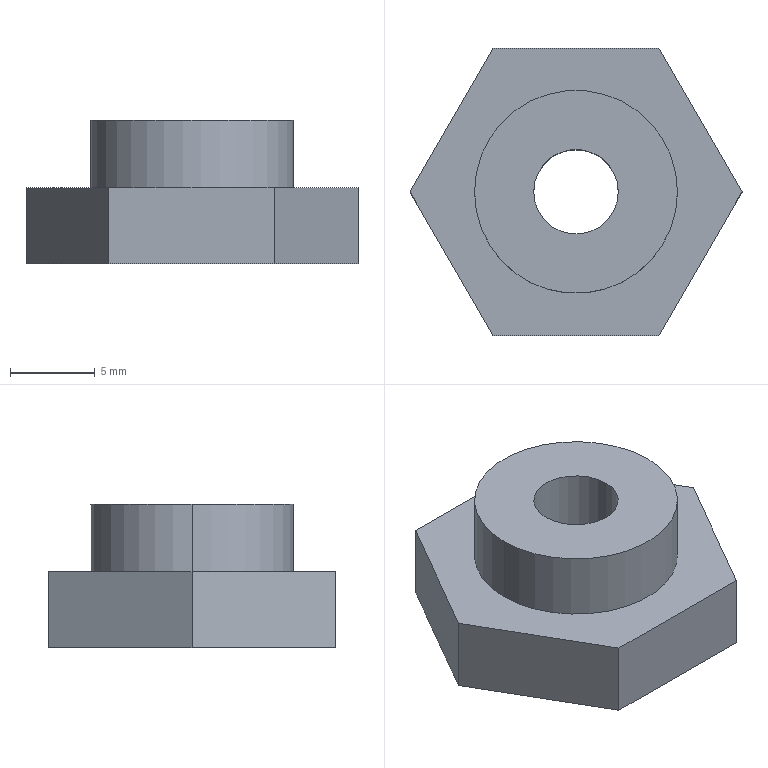Part | STEP file | Small pulley nut | 1 solid | 13 faces | box 19.63 x 17 x 8.5 mm | volume 1412 mm3 | plane 9 | cylinder 4 | commonest cylinder face diameters 5 x2 12 x2
STEP:
#1=CARTESIAN_POINT('',(0.,0.,0.));
#2=DIRECTION('',(0.,0.,1.));
#3=DIRECTION('',(1.,0.,0.));
#4=AXIS2_PLACEMENT_3D('',#1,#2,#3);
#5=CARTESIAN_POINT('',(2.5,0.,0.));
#6=VERTEX_POINT('',#5);
#7=CARTESIAN_POINT('',(2.5,0.,8.5));
#8=VERTEX_POINT('',#7);
#9=CARTESIAN_POINT('',(2.5,0.,8.5));
#10=DIRECTION('',(0.,0.,1.));
#11=VECTOR('',#10,1.);
#12=LINE('',#9,#11);
#13=CARTESIAN_POINT('',(0.,0.,8.5));
#14=DIRECTION('',(0.,0.,1.));
#15=DIRECTION('',(1.,0.,0.));
#16=AXIS2_PLACEMENT_3D('',#13,#14,#15);
#17=CYLINDRICAL_SURFACE('',#16,2.5);
#18=CARTESIAN_POINT('',(6.283,0.));
#19=DIRECTION('',(0.,1.));
#20=VECTOR('',#19,1.);
#21=LINE('',#18,#20);
#22=(GEOMETRIC_REPRESENTATION_CONTEXT(2)PARAMETRIC_REPRESENTATION_CONTEXT()REPRESENTATION_CONTEXT('',''));
#23=DEFINITIONAL_REPRESENTATION('',(#21),#22);
#24=PCURVE('',#17,#23);
#25=CARTESIAN_POINT('',(0.,0.,8.5));
#26=DIRECTION('',(0.,0.,1.));
#27=DIRECTION('',(1.,0.,0.));
#28=AXIS2_PLACEMENT_3D('',#25,#26,#27);
#29=CYLINDRICAL_SURFACE('',#28,2.5);
#30=CARTESIAN_POINT('',(0.,0.));
#31=DIRECTION('',(0.,1.));
#32=VECTOR('',#31,1.);
#33=LINE('',#30,#32);
#34=(GEOMETRIC_REPRESENTATION_CONTEXT(2)PARAMETRIC_REPRESENTATION_CONTEXT()REPRESENTATION_CONTEXT('',''));
#35=DEFINITIONAL_REPRESENTATION('',(#33),#34);
#36=PCURVE('',#29,#35);
#37=SURFACE_CURVE('',#12,(#24,#36),.PCURVE_S1.);
#38=EDGE_CURVE('',#6,#8,#37,.T.);
#39=ORIENTED_EDGE('',*,*,#38,.T.);
#40=CARTESIAN_POINT('',(-2.5,0.,8.5));
#41=VERTEX_POINT('',#40);
#42=CARTESIAN_POINT('',(0.,0.,8.5));
#43=DIRECTION('',(0.,0.,1.));
#44=DIRECTION('',(1.,0.,0.));
#45=AXIS2_PLACEMENT_3D('',#42,#43,#44);
#46=CIRCLE('',#45,2.5);
#47=CARTESIAN_POINT('',(0.,0.));
#48=DIRECTION('',(1.,0.));
#49=VECTOR('',#48,1.);
#50=LINE('',#47,#49);
#51=(GEOMETRIC_REPRESENTATION_CONTEXT(2)PARAMETRIC_REPRESENTATION_CONTEXT()REPRESENTATION_CONTEXT('',''));
#52=DEFINITIONAL_REPRESENTATION('',(#50),#51);
#53=PCURVE('',#17,#52);
#54=CARTESIAN_POINT('',(0.,0.,8.5));
#55=DIRECTION('',(0.,0.,1.));
#56=DIRECTION('',(1.,0.,0.));
#57=AXIS2_PLACEMENT_3D('',#54,#55,#56);
#58=PLANE('',#57);
#59=CARTESIAN_POINT('',(0.,0.));
#60=DIRECTION('',(1.,0.));
#61=AXIS2_PLACEMENT_2D('',#59,#60);
#62=CIRCLE('',#61,2.5);
#63=(GEOMETRIC_REPRESENTATION_CONTEXT(2)PARAMETRIC_REPRESENTATION_CONTEXT()REPRESENTATION_CONTEXT('',''));
#64=DEFINITIONAL_REPRESENTATION('',(#62),#63);
#65=PCURVE('',#58,#64);
#66=SURFACE_CURVE('',#46,(#53,#65),.PCURVE_S1.);
#67=EDGE_CURVE('',#41,#8,#66,.T.);
#68=ORIENTED_EDGE('',*,*,#67,.F.);
#69=CARTESIAN_POINT('',(-2.5,0.,0.));
#70=VERTEX_POINT('',#69);
#71=CARTESIAN_POINT('',(-2.5,0.,8.5));
#72=DIRECTION('',(0.,0.,1.));
#73=VECTOR('',#72,1.);
#74=LINE('',#71,#73);
#75=CARTESIAN_POINT('',(3.142,0.));
#76=DIRECTION('',(0.,1.));
#77=VECTOR('',#76,1.);
#78=LINE('',#75,#77);
#79=(GEOMETRIC_REPRESENTATION_CONTEXT(2)PARAMETRIC_REPRESENTATION_CONTEXT()REPRESENTATION_CONTEXT('',''));
#80=DEFINITIONAL_REPRESENTATION('',(#78),#79);
#81=PCURVE('',#17,#80);
#82=CARTESIAN_POINT('',(3.142,0.));
#83=DIRECTION('',(0.,1.));
#84=VECTOR('',#83,1.);
#85=LINE('',#82,#84);
#86=(GEOMETRIC_REPRESENTATION_CONTEXT(2)PARAMETRIC_REPRESENTATION_CONTEXT()REPRESENTATION_CONTEXT('',''));
#87=DEFINITIONAL_REPRESENTATION('',(#85),#86);
#88=PCURVE('',#29,#87);
#89=SURFACE_CURVE('',#74,(#81,#88),.PCURVE_S1.);
#90=EDGE_CURVE('',#70,#41,#89,.T.);
#91=ORIENTED_EDGE('',*,*,#90,.F.);
#92=CARTESIAN_POINT('',(0.,0.,0.));
#93=DIRECTION('',(0.,0.,1.));
#94=DIRECTION('',(1.,0.,0.));
#95=AXIS2_PLACEMENT_3D('',#92,#93,#94);
#96=CIRCLE('',#95,2.5);
#97=CARTESIAN_POINT('',(0.,-8.5));
#98=DIRECTION('',(1.,0.));
#99=VECTOR('',#98,1.);
#100=LINE('',#97,#99);
#101=(GEOMETRIC_REPRESENTATION_CONTEXT(2)PARAMETRIC_REPRESENTATION_CONTEXT()REPRESENTATION_CONTEXT('',''));
#102=DEFINITIONAL_REPRESENTATION('',(#100),#101);
#103=PCURVE('',#17,#102);
#104=CARTESIAN_POINT('',(0.,0.,0.));
#105=DIRECTION('',(0.,0.,1.));
#106=DIRECTION('',(1.,0.,0.));
#107=AXIS2_PLACEMENT_3D('',#104,#105,#106);
#108=PLANE('',#107);
#109=CARTESIAN_POINT('',(0.,0.));
#110=DIRECTION('',(1.,0.));
#111=AXIS2_PLACEMENT_2D('',#109,#110);
#112=CIRCLE('',#111,2.5);
#113=(GEOMETRIC_REPRESENTATION_CONTEXT(2)PARAMETRIC_REPRESENTATION_CONTEXT()REPRESENTATION_CONTEXT('',''));
#114=DEFINITIONAL_REPRESENTATION('',(#112),#113);
#115=PCURVE('',#108,#114);
#116=SURFACE_CURVE('',#96,(#103,#115),.PCURVE_S1.);
#117=EDGE_CURVE('',#70,#6,#116,.T.);
#118=ORIENTED_EDGE('',*,*,#117,.T.);
#119=EDGE_LOOP('',(#39,#68,#91,#118));
#120=FACE_BOUND('',#119,.F.);
#121=ADVANCED_FACE('',(#120),#17,.F.);
#122=CARTESIAN_POINT('',(6.,0.,8.5));
#123=VERTEX_POINT('',#122);
#124=CARTESIAN_POINT('',(-6.,0.,8.5));
#125=VERTEX_POINT('',#124);
#126=CARTESIAN_POINT('',(0.,0.,8.5));
#127=DIRECTION('',(0.,0.,1.));
#128=DIRECTION('',(1.,0.,0.));
#129=AXIS2_PLACEMENT_3D('',#126,#127,#128);
#130=CIRCLE('',#129,6.);
#131=CARTESIAN_POINT('',(0.,0.,8.5));
#132=DIRECTION('',(0.,0.,-1.));
#133=DIRECTION('',(-1.,0.,0.));
#134=AXIS2_PLACEMENT_3D('',#131,#132,#133);
#135=CYLINDRICAL_SURFACE('',#134,6.);
#136=CARTESIAN_POINT('',(3.142,0.));
#137=DIRECTION('',(-1.,0.));
#138=VECTOR('',#137,1.);
#139=LINE('',#136,#138);
#140=(GEOMETRIC_REPRESENTATION_CONTEXT(2)PARAMETRIC_REPRESENTATION_CONTEXT()REPRESENTATION_CONTEXT('',''));
#141=DEFINITIONAL_REPRESENTATION('',(#139),#140);
#142=PCURVE('',#135,#141);
#143=CARTESIAN_POINT('',(0.,0.));
#144=DIRECTION('',(1.,0.));
#145=AXIS2_PLACEMENT_2D('',#143,#144);
#146=CIRCLE('',#145,6.);
#147=(GEOMETRIC_REPRESENTATION_CONTEXT(2)PARAMETRIC_REPRESENTATION_CONTEXT()REPRESENTATION_CONTEXT('',''));
#148=DEFINITIONAL_REPRESENTATION('',(#146),#147);
#149=PCURVE('',#58,#148);
#150=SURFACE_CURVE('',#130,(#142,#149),.PCURVE_S1.);
#151=EDGE_CURVE('',#123,#125,#150,.T.);
#152=ORIENTED_EDGE('',*,*,#151,.F.);
#153=CARTESIAN_POINT('',(6.,0.,4.5));
#154=VERTEX_POINT('',#153);
#155=CARTESIAN_POINT('',(6.,0.,8.5));
#156=DIRECTION('',(0.,0.,-1.));
#157=VECTOR('',#156,1.);
#158=LINE('',#155,#157);
#159=CARTESIAN_POINT('',(3.142,0.));
#160=DIRECTION('',(0.,1.));
#161=VECTOR('',#160,1.);
#162=LINE('',#159,#161);
#163=(GEOMETRIC_REPRESENTATION_CONTEXT(2)PARAMETRIC_REPRESENTATION_CONTEXT()REPRESENTATION_CONTEXT('',''));
#164=DEFINITIONAL_REPRESENTATION('',(#162),#163);
#165=PCURVE('',#135,#164);
#166=CARTESIAN_POINT('',(0.,0.,8.5));
#167=DIRECTION('',(0.,0.,-1.));
#168=DIRECTION('',(-1.,0.,0.));
#169=AXIS2_PLACEMENT_3D('',#166,#167,#168);
#170=CYLINDRICAL_SURFACE('',#169,6.);
#171=CARTESIAN_POINT('',(3.142,0.));
#172=DIRECTION('',(0.,1.));
#173=VECTOR('',#172,1.);
#174=LINE('',#171,#173);
#175=(GEOMETRIC_REPRESENTATION_CONTEXT(2)PARAMETRIC_REPRESENTATION_CONTEXT()REPRESENTATION_CONTEXT('',''));
#176=DEFINITIONAL_REPRESENTATION('',(#174),#175);
#177=PCURVE('',#170,#176);
#178=SURFACE_CURVE('',#158,(#165,#177),.PCURVE_S1.);
#179=EDGE_CURVE('',#123,#154,#178,.T.);
#180=ORIENTED_EDGE('',*,*,#179,.T.);
#181=CARTESIAN_POINT('',(-6.,0.,4.5));
#182=VERTEX_POINT('',#181);
#183=CARTESIAN_POINT('',(0.,0.,4.5));
#184=DIRECTION('',(0.,0.,1.));
#185=DIRECTION('',(1.,0.,0.));
#186=AXIS2_PLACEMENT_3D('',#183,#184,#185);
#187=CIRCLE('',#186,6.);
#188=CARTESIAN_POINT('',(3.142,4.));
#189=DIRECTION('',(-1.,0.));
#190=VECTOR('',#189,1.);
#191=LINE('',#188,#190);
#192=(GEOMETRIC_REPRESENTATION_CONTEXT(2)PARAMETRIC_REPRESENTATION_CONTEXT()REPRESENTATION_CONTEXT('',''));
#193=DEFINITIONAL_REPRESENTATION('',(#191),#192);
#194=PCURVE('',#135,#193);
#195=CARTESIAN_POINT('',(0.,0.,4.5));
#196=DIRECTION('',(0.,0.,1.));
#197=DIRECTION('',(1.,0.,0.));
#198=AXIS2_PLACEMENT_3D('',#195,#196,#197);
#199=PLANE('',#198);
#200=CARTESIAN_POINT('',(0.,0.));
#201=DIRECTION('',(1.,0.));
#202=AXIS2_PLACEMENT_2D('',#200,#201);
#203=CIRCLE('',#202,6.);
#204=(GEOMETRIC_REPRESENTATION_CONTEXT(2)PARAMETRIC_REPRESENTATION_CONTEXT()REPRESENTATION_CONTEXT('',''));
#205=DEFINITIONAL_REPRESENTATION('',(#203),#204);
#206=PCURVE('',#199,#205);
#207=SURFACE_CURVE('',#187,(#194,#206),.PCURVE_S1.);
#208=EDGE_CURVE('',#154,#182,#207,.T.);
#209=ORIENTED_EDGE('',*,*,#208,.T.);
#210=CARTESIAN_POINT('',(-6.,0.,8.5));
#211=DIRECTION('',(0.,0.,-1.));
#212=VECTOR('',#211,1.);
#213=LINE('',#210,#212);
#214=CARTESIAN_POINT('',(0.,0.));
#215=DIRECTION('',(0.,1.));
#216=VECTOR('',#215,1.);
#217=LINE('',#214,#216);
#218=(GEOMETRIC_REPRESENTATION_CONTEXT(2)PARAMETRIC_REPRESENTATION_CONTEXT()REPRESENTATION_CONTEXT('',''));
#219=DEFINITIONAL_REPRESENTATION('',(#217),#218);
#220=PCURVE('',#135,#219);
#221=CARTESIAN_POINT('',(6.283,0.));
#222=DIRECTION('',(0.,1.));
#223=VECTOR('',#222,1.);
#224=LINE('',#221,#223);
#225=(GEOMETRIC_REPRESENTATION_CONTEXT(2)PARAMETRIC_REPRESENTATION_CONTEXT()REPRESENTATION_CONTEXT('',''));
#226=DEFINITIONAL_REPRESENTATION('',(#224),#225);
#227=PCURVE('',#170,#226);
#228=SURFACE_CURVE('',#213,(#220,#227),.PCURVE_S1.);
#229=EDGE_CURVE('',#125,#182,#228,.T.);
#230=ORIENTED_EDGE('',*,*,#229,.F.);
#231=EDGE_LOOP('',(#152,#180,#209,#230));
#232=FACE_BOUND('',#231,.T.);
#233=ADVANCED_FACE('',(#232),#135,.T.);
#234=CARTESIAN_POINT('',(4.907,-8.5,0.));
#235=VERTEX_POINT('',#234);
#236=CARTESIAN_POINT('',(9.815,0.,0.));
#237=VERTEX_POINT('',#236);
#238=CARTESIAN_POINT('',(4.907,-8.5,0.));
#239=DIRECTION('',(0.5,0.866,0.));
#240=VECTOR('',#239,1.);
#241=LINE('',#238,#240);
#242=CARTESIAN_POINT('',(4.907,-8.5,4.5));
#243=DIRECTION('',(-0.866,0.5,0.));
#244=DIRECTION('',(-0.5,-0.866,0.));
#245=AXIS2_PLACEMENT_3D('',#242,#243,#244);
#246=PLANE('',#245);
#247=CARTESIAN_POINT('',(0.,-4.5));
#248=DIRECTION('',(-1.,0.));
#249=VECTOR('',#248,1.);
#250=LINE('',#247,#249);
#251=(GEOMETRIC_REPRESENTATION_CONTEXT(2)PARAMETRIC_REPRESENTATION_CONTEXT()REPRESENTATION_CONTEXT('',''));
#252=DEFINITIONAL_REPRESENTATION('',(#250),#251);
#253=PCURVE('',#246,#252);
#254=CARTESIAN_POINT('',(4.907,-8.5));
#255=DIRECTION('',(0.5,0.866));
#256=VECTOR('',#255,1.);
#257=LINE('',#254,#256);
#258=(GEOMETRIC_REPRESENTATION_CONTEXT(2)PARAMETRIC_REPRESENTATION_CONTEXT()REPRESENTATION_CONTEXT('',''));
#259=DEFINITIONAL_REPRESENTATION('',(#257),#258);
#260=PCURVE('',#108,#259);
#261=SURFACE_CURVE('',#241,(#253,#260),.PCURVE_S1.);
#262=EDGE_CURVE('',#235,#237,#261,.T.);
#263=ORIENTED_EDGE('',*,*,#262,.T.);
#264=CARTESIAN_POINT('',(9.815,0.,4.5));
#265=VERTEX_POINT('',#264);
#266=CARTESIAN_POINT('',(9.815,0.,4.5));
#267=DIRECTION('',(0.,0.,-1.));
#268=VECTOR('',#267,1.);
#269=LINE('',#266,#268);
#270=CARTESIAN_POINT('',(-9.815,0.));
#271=DIRECTION('',(0.,-1.));
#272=VECTOR('',#271,1.);
#273=LINE('',#270,#272);
#274=(GEOMETRIC_REPRESENTATION_CONTEXT(2)PARAMETRIC_REPRESENTATION_CONTEXT()REPRESENTATION_CONTEXT('',''));
#275=DEFINITIONAL_REPRESENTATION('',(#273),#274);
#276=PCURVE('',#246,#275);
#277=CARTESIAN_POINT('',(9.815,0.,4.5));
#278=DIRECTION('',(-0.866,-0.5,0.));
#279=DIRECTION('',(0.5,-0.866,0.));
#280=AXIS2_PLACEMENT_3D('',#277,#278,#279);
#281=PLANE('',#280);
#282=CARTESIAN_POINT('',(0.,0.));
#283=DIRECTION('',(0.,-1.));
#284=VECTOR('',#283,1.);
#285=LINE('',#282,#284);
#286=(GEOMETRIC_REPRESENTATION_CONTEXT(2)PARAMETRIC_REPRESENTATION_CONTEXT()REPRESENTATION_CONTEXT('',''));
#287=DEFINITIONAL_REPRESENTATION('',(#285),#286);
#288=PCURVE('',#281,#287);
#289=SURFACE_CURVE('',#269,(#276,#288),.PCURVE_S1.);
#290=EDGE_CURVE('',#265,#237,#289,.T.);
#291=ORIENTED_EDGE('',*,*,#290,.F.);
#292=CARTESIAN_POINT('',(4.907,-8.5,4.5));
#293=VERTEX_POINT('',#292);
#294=CARTESIAN_POINT('',(4.907,-8.5,4.5));
#295=DIRECTION('',(0.5,0.866,0.));
#296=VECTOR('',#295,1.);
#297=LINE('',#294,#296);
#298=CARTESIAN_POINT('',(0.,0.));
#299=DIRECTION('',(-1.,0.));
#300=VECTOR('',#299,1.);
#301=LINE('',#298,#300);
#302=(GEOMETRIC_REPRESENTATION_CONTEXT(2)PARAMETRIC_REPRESENTATION_CONTEXT()REPRESENTATION_CONTEXT('',''));
#303=DEFINITIONAL_REPRESENTATION('',(#301),#302);
#304=PCURVE('',#246,#303);
#305=CARTESIAN_POINT('',(4.907,-8.5));
#306=DIRECTION('',(0.5,0.866));
#307=VECTOR('',#306,1.);
#308=LINE('',#305,#307);
#309=(GEOMETRIC_REPRESENTATION_CONTEXT(2)PARAMETRIC_REPRESENTATION_CONTEXT()REPRESENTATION_CONTEXT('',''));
#310=DEFINITIONAL_REPRESENTATION('',(#308),#309);
#311=PCURVE('',#199,#310);
#312=SURFACE_CURVE('',#297,(#304,#311),.PCURVE_S1.);
#313=EDGE_CURVE('',#293,#265,#312,.T.);
#314=ORIENTED_EDGE('',*,*,#313,.F.);
#315=CARTESIAN_POINT('',(4.907,-8.5,4.5));
#316=DIRECTION('',(0.,0.,-1.));
#317=VECTOR('',#316,1.);
#318=LINE('',#315,#317);
#319=CARTESIAN_POINT('',(0.,0.));
#320=DIRECTION('',(0.,-1.));
#321=VECTOR('',#320,1.);
#322=LINE('',#319,#321);
#323=(GEOMETRIC_REPRESENTATION_CONTEXT(2)PARAMETRIC_REPRESENTATION_CONTEXT()REPRESENTATION_CONTEXT('',''));
#324=DEFINITIONAL_REPRESENTATION('',(#322),#323);
#325=PCURVE('',#246,#324);
#326=CARTESIAN_POINT('',(-4.907,-8.5,4.5));
#327=DIRECTION('',(0.,1.,0.));
#328=DIRECTION('',(-1.,0.,0.));
#329=AXIS2_PLACEMENT_3D('',#326,#327,#328);
#330=PLANE('',#329);
#331=CARTESIAN_POINT('',(-9.815,0.));
#332=DIRECTION('',(0.,-1.));
#333=VECTOR('',#332,1.);
#334=LINE('',#331,#333);
#335=(GEOMETRIC_REPRESENTATION_CONTEXT(2)PARAMETRIC_REPRESENTATION_CONTEXT()REPRESENTATION_CONTEXT('',''));
#336=DEFINITIONAL_REPRESENTATION('',(#334),#335);
#337=PCURVE('',#330,#336);
#338=SURFACE_CURVE('',#318,(#325,#337),.PCURVE_S1.);
#339=EDGE_CURVE('',#293,#235,#338,.T.);
#340=ORIENTED_EDGE('',*,*,#339,.T.);
#341=EDGE_LOOP('',(#263,#291,#314,#340));
#342=FACE_BOUND('',#341,.T.);
#343=ADVANCED_FACE('',(#342),#246,.F.);
#344=CARTESIAN_POINT('',(4.907,8.5,0.));
#345=VERTEX_POINT('',#344);
#346=CARTESIAN_POINT('',(9.815,0.,0.));
#347=DIRECTION('',(-0.5,0.866,0.));
#348=VECTOR('',#347,1.);
#349=LINE('',#346,#348);
#350=CARTESIAN_POINT('',(0.,-4.5));
#351=DIRECTION('',(-1.,0.));
#352=VECTOR('',#351,1.);
#353=LINE('',#350,#352);
#354=(GEOMETRIC_REPRESENTATION_CONTEXT(2)PARAMETRIC_REPRESENTATION_CONTEXT()REPRESENTATION_CONTEXT('',''));
#355=DEFINITIONAL_REPRESENTATION('',(#353),#354);
#356=PCURVE('',#281,#355);
#357=CARTESIAN_POINT('',(9.815,0.));
#358=DIRECTION('',(-0.5,0.866));
#359=VECTOR('',#358,1.);
#360=LINE('',#357,#359);
#361=(GEOMETRIC_REPRESENTATION_CONTEXT(2)PARAMETRIC_REPRESENTATION_CONTEXT()REPRESENTATION_CONTEXT('',''));
#362=DEFINITIONAL_REPRESENTATION('',(#360),#361);
#363=PCURVE('',#108,#362);
#364=SURFACE_CURVE('',#349,(#356,#363),.PCURVE_S1.);
#365=EDGE_CURVE('',#237,#345,#364,.T.);
#366=ORIENTED_EDGE('',*,*,#365,.T.);
#367=CARTESIAN_POINT('',(4.907,8.5,4.5));
#368=VERTEX_POINT('',#367);
#369=CARTESIAN_POINT('',(4.907,8.5,4.5));
#370=DIRECTION('',(0.,0.,-1.));
#371=VECTOR('',#370,1.);
#372=LINE('',#369,#371);
#373=CARTESIAN_POINT('',(-9.815,0.));
#374=DIRECTION('',(0.,-1.));
#375=VECTOR('',#374,1.);
#376=LINE('',#373,#375);
#377=(GEOMETRIC_REPRESENTATION_CONTEXT(2)PARAMETRIC_REPRESENTATION_CONTEXT()REPRESENTATION_CONTEXT('',''));
#378=DEFINITIONAL_REPRESENTATION('',(#376),#377);
#379=PCURVE('',#281,#378);
#380=CARTESIAN_POINT('',(4.907,8.5,4.5));
#381=DIRECTION('',(0.,-1.,0.));
#382=DIRECTION('',(1.,0.,0.));
#383=AXIS2_PLACEMENT_3D('',#380,#381,#382);
#384=PLANE('',#383);
#385=CARTESIAN_POINT('',(0.,0.));
#386=DIRECTION('',(0.,-1.));
#387=VECTOR('',#386,1.);
#388=LINE('',#385,#387);
#389=(GEOMETRIC_REPRESENTATION_CONTEXT(2)PARAMETRIC_REPRESENTATION_CONTEXT()REPRESENTATION_CONTEXT('',''));
#390=DEFINITIONAL_REPRESENTATION('',(#388),#389);
#391=PCURVE('',#384,#390);
#392=SURFACE_CURVE('',#372,(#379,#391),.PCURVE_S1.);
#393=EDGE_CURVE('',#368,#345,#392,.T.);
#394=ORIENTED_EDGE('',*,*,#393,.F.);
#395=CARTESIAN_POINT('',(9.815,0.,4.5));
#396=DIRECTION('',(-0.5,0.866,0.));
#397=VECTOR('',#396,1.);
#398=LINE('',#395,#397);
#399=CARTESIAN_POINT('',(0.,0.));
#400=DIRECTION('',(-1.,0.));
#401=VECTOR('',#400,1.);
#402=LINE('',#399,#401);
#403=(GEOMETRIC_REPRESENTATION_CONTEXT(2)PARAMETRIC_REPRESENTATION_CONTEXT()REPRESENTATION_CONTEXT('',''));
#404=DEFINITIONAL_REPRESENTATION('',(#402),#403);
#405=PCURVE('',#281,#404);
#406=CARTESIAN_POINT('',(9.815,0.));
#407=DIRECTION('',(-0.5,0.866));
#408=VECTOR('',#407,1.);
#409=LINE('',#406,#408);
#410=(GEOMETRIC_REPRESENTATION_CONTEXT(2)PARAMETRIC_REPRESENTATION_CONTEXT()REPRESENTATION_CONTEXT('',''));
#411=DEFINITIONAL_REPRESENTATION('',(#409),#410);
#412=PCURVE('',#199,#411);
#413=SURFACE_CURVE('',#398,(#405,#412),.PCURVE_S1.);
#414=EDGE_CURVE('',#265,#368,#413,.T.);
#415=ORIENTED_EDGE('',*,*,#414,.F.);
#416=ORIENTED_EDGE('',*,*,#290,.T.);
#417=EDGE_LOOP('',(#366,#394,#415,#416));
#418=FACE_BOUND('',#417,.T.);
#419=ADVANCED_FACE('',(#418),#281,.F.);
#420=CARTESIAN_POINT('',(-4.907,8.5,0.));
#421=VERTEX_POINT('',#420);
#422=CARTESIAN_POINT('',(4.907,8.5,0.));
#423=DIRECTION('',(-1.,0.,0.));
#424=VECTOR('',#423,1.);
#425=LINE('',#422,#424);
#426=CARTESIAN_POINT('',(0.,-4.5));
#427=DIRECTION('',(-1.,0.));
#428=VECTOR('',#427,1.);
#429=LINE('',#426,#428);
#430=(GEOMETRIC_REPRESENTATION_CONTEXT(2)PARAMETRIC_REPRESENTATION_CONTEXT()REPRESENTATION_CONTEXT('',''));
#431=DEFINITIONAL_REPRESENTATION('',(#429),#430);
#432=PCURVE('',#384,#431);
#433=CARTESIAN_POINT('',(4.907,8.5));
#434=DIRECTION('',(-1.,0.));
#435=VECTOR('',#434,1.);
#436=LINE('',#433,#435);
#437=(GEOMETRIC_REPRESENTATION_CONTEXT(2)PARAMETRIC_REPRESENTATION_CONTEXT()REPRESENTATION_CONTEXT('',''));
#438=DEFINITIONAL_REPRESENTATION('',(#436),#437);
#439=PCURVE('',#108,#438);
#440=SURFACE_CURVE('',#425,(#432,#439),.PCURVE_S1.);
#441=EDGE_CURVE('',#345,#421,#440,.T.);
#442=ORIENTED_EDGE('',*,*,#441,.T.);
#443=CARTESIAN_POINT('',(-4.907,8.5,4.5));
#444=VERTEX_POINT('',#443);
#445=CARTESIAN_POINT('',(-4.907,8.5,4.5));
#446=DIRECTION('',(0.,0.,-1.));
#447=VECTOR('',#446,1.);
#448=LINE('',#445,#447);
#449=CARTESIAN_POINT('',(-9.815,0.));
#450=DIRECTION('',(0.,-1.));
#451=VECTOR('',#450,1.);
#452=LINE('',#449,#451);
#453=(GEOMETRIC_REPRESENTATION_CONTEXT(2)PARAMETRIC_REPRESENTATION_CONTEXT()REPRESENTATION_CONTEXT('',''));
#454=DEFINITIONAL_REPRESENTATION('',(#452),#453);
#455=PCURVE('',#384,#454);
#456=CARTESIAN_POINT('',(-4.907,8.5,4.5));
#457=DIRECTION('',(0.866,-0.5,0.));
#458=DIRECTION('',(0.5,0.866,0.));
#459=AXIS2_PLACEMENT_3D('',#456,#457,#458);
#460=PLANE('',#459);
#461=CARTESIAN_POINT('',(0.,0.));
#462=DIRECTION('',(0.,-1.));
#463=VECTOR('',#462,1.);
#464=LINE('',#461,#463);
#465=(GEOMETRIC_REPRESENTATION_CONTEXT(2)PARAMETRIC_REPRESENTATION_CONTEXT()REPRESENTATION_CONTEXT('',''));
#466=DEFINITIONAL_REPRESENTATION('',(#464),#465);
#467=PCURVE('',#460,#466);
#468=SURFACE_CURVE('',#448,(#455,#467),.PCURVE_S1.);
#469=EDGE_CURVE('',#444,#421,#468,.T.);
#470=ORIENTED_EDGE('',*,*,#469,.F.);
#471=CARTESIAN_POINT('',(4.907,8.5,4.5));
#472=DIRECTION('',(-1.,0.,0.));
#473=VECTOR('',#472,1.);
#474=LINE('',#471,#473);
#475=CARTESIAN_POINT('',(0.,0.));
#476=DIRECTION('',(-1.,0.));
#477=VECTOR('',#476,1.);
#478=LINE('',#475,#477);
#479=(GEOMETRIC_REPRESENTATION_CONTEXT(2)PARAMETRIC_REPRESENTATION_CONTEXT()REPRESENTATION_CONTEXT('',''));
#480=DEFINITIONAL_REPRESENTATION('',(#478),#479);
#481=PCURVE('',#384,#480);
#482=CARTESIAN_POINT('',(4.907,8.5));
#483=DIRECTION('',(-1.,0.));
#484=VECTOR('',#483,1.);
#485=LINE('',#482,#484);
#486=(GEOMETRIC_REPRESENTATION_CONTEXT(2)PARAMETRIC_REPRESENTATION_CONTEXT()REPRESENTATION_CONTEXT('',''));
#487=DEFINITIONAL_REPRESENTATION('',(#485),#486);
#488=PCURVE('',#199,#487);
#489=SURFACE_CURVE('',#474,(#481,#488),.PCURVE_S1.);
#490=EDGE_CURVE('',#368,#444,#489,.T.);
#491=ORIENTED_EDGE('',*,*,#490,.F.);
#492=ORIENTED_EDGE('',*,*,#393,.T.);
#493=EDGE_LOOP('',(#442,#470,#491,#492));
#494=FACE_BOUND('',#493,.T.);
#495=ADVANCED_FACE('',(#494),#384,.F.);
#496=CARTESIAN_POINT('',(-9.815,0.,0.));
#497=VERTEX_POINT('',#496);
#498=CARTESIAN_POINT('',(-4.907,8.5,0.));
#499=DIRECTION('',(-0.5,-0.866,0.));
#500=VECTOR('',#499,1.);
#501=LINE('',#498,#500);
#502=CARTESIAN_POINT('',(0.,-4.5));
#503=DIRECTION('',(-1.,0.));
#504=VECTOR('',#503,1.);
#505=LINE('',#502,#504);
#506=(GEOMETRIC_REPRESENTATION_CONTEXT(2)PARAMETRIC_REPRESENTATION_CONTEXT()REPRESENTATION_CONTEXT('',''));
#507=DEFINITIONAL_REPRESENTATION('',(#505),#506);
#508=PCURVE('',#460,#507);
#509=CARTESIAN_POINT('',(-4.907,8.5));
#510=DIRECTION('',(-0.5,-0.866));
#511=VECTOR('',#510,1.);
#512=LINE('',#509,#511);
#513=(GEOMETRIC_REPRESENTATION_CONTEXT(2)PARAMETRIC_REPRESENTATION_CONTEXT()REPRESENTATION_CONTEXT('',''));
#514=DEFINITIONAL_REPRESENTATION('',(#512),#513);
#515=PCURVE('',#108,#514);
#516=SURFACE_CURVE('',#501,(#508,#515),.PCURVE_S1.);
#517=EDGE_CURVE('',#421,#497,#516,.T.);
#518=ORIENTED_EDGE('',*,*,#517,.T.);
#519=CARTESIAN_POINT('',(-9.815,0.,4.5));
#520=VERTEX_POINT('',#519);
#521=CARTESIAN_POINT('',(-9.815,0.,4.5));
#522=DIRECTION('',(0.,0.,-1.));
#523=VECTOR('',#522,1.);
#524=LINE('',#521,#523);
#525=CARTESIAN_POINT('',(-9.815,0.));
#526=DIRECTION('',(0.,-1.));
#527=VECTOR('',#526,1.);
#528=LINE('',#525,#527);
#529=(GEOMETRIC_REPRESENTATION_CONTEXT(2)PARAMETRIC_REPRESENTATION_CONTEXT()REPRESENTATION_CONTEXT('',''));
#530=DEFINITIONAL_REPRESENTATION('',(#528),#529);
#531=PCURVE('',#460,#530);
#532=CARTESIAN_POINT('',(-9.815,0.,4.5));
#533=DIRECTION('',(0.866,0.5,0.));
#534=DIRECTION('',(-0.5,0.866,0.));
#535=AXIS2_PLACEMENT_3D('',#532,#533,#534);
#536=PLANE('',#535);
#537=CARTESIAN_POINT('',(0.,0.));
#538=DIRECTION('',(0.,-1.));
#539=VECTOR('',#538,1.);
#540=LINE('',#537,#539);
#541=(GEOMETRIC_REPRESENTATION_CONTEXT(2)PARAMETRIC_REPRESENTATION_CONTEXT()REPRESENTATION_CONTEXT('',''));
#542=DEFINITIONAL_REPRESENTATION('',(#540),#541);
#543=PCURVE('',#536,#542);
#544=SURFACE_CURVE('',#524,(#531,#543),.PCURVE_S1.);
#545=EDGE_CURVE('',#520,#497,#544,.T.);
#546=ORIENTED_EDGE('',*,*,#545,.F.);
#547=CARTESIAN_POINT('',(-4.907,8.5,4.5));
#548=DIRECTION('',(-0.5,-0.866,0.));
#549=VECTOR('',#548,1.);
#550=LINE('',#547,#549);
#551=CARTESIAN_POINT('',(0.,0.));
#552=DIRECTION('',(-1.,0.));
#553=VECTOR('',#552,1.);
#554=LINE('',#551,#553);
#555=(GEOMETRIC_REPRESENTATION_CONTEXT(2)PARAMETRIC_REPRESENTATION_CONTEXT()REPRESENTATION_CONTEXT('',''));
#556=DEFINITIONAL_REPRESENTATION('',(#554),#555);
#557=PCURVE('',#460,#556);
#558=CARTESIAN_POINT('',(-4.907,8.5));
#559=DIRECTION('',(-0.5,-0.866));
#560=VECTOR('',#559,1.);
#561=LINE('',#558,#560);
#562=(GEOMETRIC_REPRESENTATION_CONTEXT(2)PARAMETRIC_REPRESENTATION_CONTEXT()REPRESENTATION_CONTEXT('',''));
#563=DEFINITIONAL_REPRESENTATION('',(#561),#562);
#564=PCURVE('',#199,#563);
#565=SURFACE_CURVE('',#550,(#557,#564),.PCURVE_S1.);
#566=EDGE_CURVE('',#444,#520,#565,.T.);
#567=ORIENTED_EDGE('',*,*,#566,.F.);
#568=ORIENTED_EDGE('',*,*,#469,.T.);
#569=EDGE_LOOP('',(#518,#546,#567,#568));
#570=FACE_BOUND('',#569,.T.);
#571=ADVANCED_FACE('',(#570),#460,.F.);
#572=CARTESIAN_POINT('',(-4.907,-8.5,0.));
#573=VERTEX_POINT('',#572);
#574=CARTESIAN_POINT('',(-9.815,0.,0.));
#575=DIRECTION('',(0.5,-0.866,0.));
#576=VECTOR('',#575,1.);
#577=LINE('',#574,#576);
#578=CARTESIAN_POINT('',(0.,-4.5));
#579=DIRECTION('',(-1.,0.));
#580=VECTOR('',#579,1.);
#581=LINE('',#578,#580);
#582=(GEOMETRIC_REPRESENTATION_CONTEXT(2)PARAMETRIC_REPRESENTATION_CONTEXT()REPRESENTATION_CONTEXT('',''));
#583=DEFINITIONAL_REPRESENTATION('',(#581),#582);
#584=PCURVE('',#536,#583);
#585=CARTESIAN_POINT('',(-9.815,0.));
#586=DIRECTION('',(0.5,-0.866));
#587=VECTOR('',#586,1.);
#588=LINE('',#585,#587);
#589=(GEOMETRIC_REPRESENTATION_CONTEXT(2)PARAMETRIC_REPRESENTATION_CONTEXT()REPRESENTATION_CONTEXT('',''));
#590=DEFINITIONAL_REPRESENTATION('',(#588),#589);
#591=PCURVE('',#108,#590);
#592=SURFACE_CURVE('',#577,(#584,#591),.PCURVE_S1.);
#593=EDGE_CURVE('',#497,#573,#592,.T.);
#594=ORIENTED_EDGE('',*,*,#593,.T.);
#595=CARTESIAN_POINT('',(-4.907,-8.5,4.5));
#596=VERTEX_POINT('',#595);
#597=CARTESIAN_POINT('',(-4.907,-8.5,4.5));
#598=DIRECTION('',(0.,0.,-1.));
#599=VECTOR('',#598,1.);
#600=LINE('',#597,#599);
#601=CARTESIAN_POINT('',(-9.815,0.));
#602=DIRECTION('',(0.,-1.));
#603=VECTOR('',#602,1.);
#604=LINE('',#601,#603);
#605=(GEOMETRIC_REPRESENTATION_CONTEXT(2)PARAMETRIC_REPRESENTATION_CONTEXT()REPRESENTATION_CONTEXT('',''));
#606=DEFINITIONAL_REPRESENTATION('',(#604),#605);
#607=PCURVE('',#536,#606);
#608=CARTESIAN_POINT('',(0.,0.));
#609=DIRECTION('',(0.,-1.));
#610=VECTOR('',#609,1.);
#611=LINE('',#608,#610);
#612=(GEOMETRIC_REPRESENTATION_CONTEXT(2)PARAMETRIC_REPRESENTATION_CONTEXT()REPRESENTATION_CONTEXT('',''));
#613=DEFINITIONAL_REPRESENTATION('',(#611),#612);
#614=PCURVE('',#330,#613);
#615=SURFACE_CURVE('',#600,(#607,#614),.PCURVE_S1.);
#616=EDGE_CURVE('',#596,#573,#615,.T.);
#617=ORIENTED_EDGE('',*,*,#616,.F.);
#618=CARTESIAN_POINT('',(-9.815,0.,4.5));
#619=DIRECTION('',(0.5,-0.866,0.));
#620=VECTOR('',#619,1.);
#621=LINE('',#618,#620);
#622=CARTESIAN_POINT('',(0.,0.));
#623=DIRECTION('',(-1.,0.));
#624=VECTOR('',#623,1.);
#625=LINE('',#622,#624);
#626=(GEOMETRIC_REPRESENTATION_CONTEXT(2)PARAMETRIC_REPRESENTATION_CONTEXT()REPRESENTATION_CONTEXT('',''));
#627=DEFINITIONAL_REPRESENTATION('',(#625),#626);
#628=PCURVE('',#536,#627);
#629=CARTESIAN_POINT('',(-9.815,0.));
#630=DIRECTION('',(0.5,-0.866));
#631=VECTOR('',#630,1.);
#632=LINE('',#629,#631);
#633=(GEOMETRIC_REPRESENTATION_CONTEXT(2)PARAMETRIC_REPRESENTATION_CONTEXT()REPRESENTATION_CONTEXT('',''));
#634=DEFINITIONAL_REPRESENTATION('',(#632),#633);
#635=PCURVE('',#199,#634);
#636=SURFACE_CURVE('',#621,(#628,#635),.PCURVE_S1.);
#637=EDGE_CURVE('',#520,#596,#636,.T.);
#638=ORIENTED_EDGE('',*,*,#637,.F.);
#639=ORIENTED_EDGE('',*,*,#545,.T.);
#640=EDGE_LOOP('',(#594,#617,#638,#639));
#641=FACE_BOUND('',#640,.T.);
#642=ADVANCED_FACE('',(#641),#536,.F.);
#643=CARTESIAN_POINT('',(-4.907,-8.5,0.));
#644=DIRECTION('',(1.,0.,0.));
#645=VECTOR('',#644,1.);
#646=LINE('',#643,#645);
#647=CARTESIAN_POINT('',(0.,-4.5));
#648=DIRECTION('',(-1.,0.));
#649=VECTOR('',#648,1.);
#650=LINE('',#647,#649);
#651=(GEOMETRIC_REPRESENTATION_CONTEXT(2)PARAMETRIC_REPRESENTATION_CONTEXT()REPRESENTATION_CONTEXT('',''));
#652=DEFINITIONAL_REPRESENTATION('',(#650),#651);
#653=PCURVE('',#330,#652);
#654=CARTESIAN_POINT('',(-4.907,-8.5));
#655=DIRECTION('',(1.,0.));
#656=VECTOR('',#655,1.);
#657=LINE('',#654,#656);
#658=(GEOMETRIC_REPRESENTATION_CONTEXT(2)PARAMETRIC_REPRESENTATION_CONTEXT()REPRESENTATION_CONTEXT('',''));
#659=DEFINITIONAL_REPRESENTATION('',(#657),#658);
#660=PCURVE('',#108,#659);
#661=SURFACE_CURVE('',#646,(#653,#660),.PCURVE_S1.);
#662=EDGE_CURVE('',#573,#235,#661,.T.);
#663=ORIENTED_EDGE('',*,*,#662,.T.);
#664=ORIENTED_EDGE('',*,*,#339,.F.);
#665=CARTESIAN_POINT('',(-4.907,-8.5,4.5));
#666=DIRECTION('',(1.,0.,0.));
#667=VECTOR('',#666,1.);
#668=LINE('',#665,#667);
#669=CARTESIAN_POINT('',(0.,0.));
#670=DIRECTION('',(-1.,0.));
#671=VECTOR('',#670,1.);
#672=LINE('',#669,#671);
#673=(GEOMETRIC_REPRESENTATION_CONTEXT(2)PARAMETRIC_REPRESENTATION_CONTEXT()REPRESENTATION_CONTEXT('',''));
#674=DEFINITIONAL_REPRESENTATION('',(#672),#673);
#675=PCURVE('',#330,#674);
#676=CARTESIAN_POINT('',(-4.907,-8.5));
#677=DIRECTION('',(1.,0.));
#678=VECTOR('',#677,1.);
#679=LINE('',#676,#678);
#680=(GEOMETRIC_REPRESENTATION_CONTEXT(2)PARAMETRIC_REPRESENTATION_CONTEXT()REPRESENTATION_CONTEXT('',''));
#681=DEFINITIONAL_REPRESENTATION('',(#679),#680);
#682=PCURVE('',#199,#681);
#683=SURFACE_CURVE('',#668,(#675,#682),.PCURVE_S1.);
#684=EDGE_CURVE('',#596,#293,#683,.T.);
#685=ORIENTED_EDGE('',*,*,#684,.F.);
#686=ORIENTED_EDGE('',*,*,#616,.T.);
#687=EDGE_LOOP('',(#663,#664,#685,#686));
#688=FACE_BOUND('',#687,.T.);
#689=ADVANCED_FACE('',(#688),#330,.F.);
#690=CARTESIAN_POINT('',(0.,0.,4.5));
#691=DIRECTION('',(0.,0.,1.));
#692=DIRECTION('',(1.,0.,0.));
#693=AXIS2_PLACEMENT_3D('',#690,#691,#692);
#694=CIRCLE('',#693,6.);
#695=CARTESIAN_POINT('',(0.,0.));
#696=DIRECTION('',(1.,0.));
#697=AXIS2_PLACEMENT_2D('',#695,#696);
#698=CIRCLE('',#697,6.);
#699=(GEOMETRIC_REPRESENTATION_CONTEXT(2)PARAMETRIC_REPRESENTATION_CONTEXT()REPRESENTATION_CONTEXT('',''));
#700=DEFINITIONAL_REPRESENTATION('',(#698),#699);
#701=PCURVE('',#199,#700);
#702=CARTESIAN_POINT('',(9.425,4.));
#703=DIRECTION('',(-1.,0.));
#704=VECTOR('',#703,1.);
#705=LINE('',#702,#704);
#706=(GEOMETRIC_REPRESENTATION_CONTEXT(2)PARAMETRIC_REPRESENTATION_CONTEXT()REPRESENTATION_CONTEXT('',''));
#707=DEFINITIONAL_REPRESENTATION('',(#705),#706);
#708=PCURVE('',#170,#707);
#709=SURFACE_CURVE('',#694,(#701,#708),.PCURVE_S1.);
#710=EDGE_CURVE('',#182,#154,#709,.T.);
#711=ORIENTED_EDGE('',*,*,#710,.F.);
#712=ORIENTED_EDGE('',*,*,#208,.F.);
#713=EDGE_LOOP('',(#711,#712));
#714=FACE_BOUND('',#713,.T.);
#715=ORIENTED_EDGE('',*,*,#313,.T.);
#716=ORIENTED_EDGE('',*,*,#414,.T.);
#717=ORIENTED_EDGE('',*,*,#490,.T.);
#718=ORIENTED_EDGE('',*,*,#566,.T.);
#719=ORIENTED_EDGE('',*,*,#637,.T.);
#720=ORIENTED_EDGE('',*,*,#684,.T.);
#721=EDGE_LOOP('',(#715,#716,#717,#718,#719,#720));
#722=FACE_BOUND('',#721,.T.);
#723=ADVANCED_FACE('',(#714,#722),#199,.T.);
#724=CARTESIAN_POINT('',(0.,0.,0.));
#725=DIRECTION('',(0.,0.,1.));
#726=DIRECTION('',(1.,0.,0.));
#727=AXIS2_PLACEMENT_3D('',#724,#725,#726);
#728=CIRCLE('',#727,2.5);
#729=CARTESIAN_POINT('',(0.,0.));
#730=DIRECTION('',(1.,0.));
#731=AXIS2_PLACEMENT_2D('',#729,#730);
#732=CIRCLE('',#731,2.5);
#733=(GEOMETRIC_REPRESENTATION_CONTEXT(2)PARAMETRIC_REPRESENTATION_CONTEXT()REPRESENTATION_CONTEXT('',''));
#734=DEFINITIONAL_REPRESENTATION('',(#732),#733);
#735=PCURVE('',#108,#734);
#736=CARTESIAN_POINT('',(0.,-8.5));
#737=DIRECTION('',(1.,0.));
#738=VECTOR('',#737,1.);
#739=LINE('',#736,#738);
#740=(GEOMETRIC_REPRESENTATION_CONTEXT(2)PARAMETRIC_REPRESENTATION_CONTEXT()REPRESENTATION_CONTEXT('',''));
#741=DEFINITIONAL_REPRESENTATION('',(#739),#740);
#742=PCURVE('',#29,#741);
#743=SURFACE_CURVE('',#728,(#735,#742),.PCURVE_S1.);
#744=EDGE_CURVE('',#6,#70,#743,.T.);
#745=ORIENTED_EDGE('',*,*,#744,.T.);
#746=ORIENTED_EDGE('',*,*,#117,.T.);
#747=EDGE_LOOP('',(#745,#746));
#748=FACE_BOUND('',#747,.T.);
#749=ORIENTED_EDGE('',*,*,#262,.F.);
#750=ORIENTED_EDGE('',*,*,#662,.F.);
#751=ORIENTED_EDGE('',*,*,#593,.F.);
#752=ORIENTED_EDGE('',*,*,#517,.F.);
#753=ORIENTED_EDGE('',*,*,#441,.F.);
#754=ORIENTED_EDGE('',*,*,#365,.F.);
#755=EDGE_LOOP('',(#749,#750,#751,#752,#753,#754));
#756=FACE_BOUND('',#755,.T.);
#757=ADVANCED_FACE('',(#748,#756),#108,.F.);
#758=ORIENTED_EDGE('',*,*,#179,.F.);
#759=CARTESIAN_POINT('',(0.,0.,8.5));
#760=DIRECTION('',(0.,0.,1.));
#761=DIRECTION('',(1.,0.,0.));
#762=AXIS2_PLACEMENT_3D('',#759,#760,#761);
#763=CIRCLE('',#762,6.);
#764=CARTESIAN_POINT('',(9.425,0.));
#765=DIRECTION('',(-1.,0.));
#766=VECTOR('',#765,1.);
#767=LINE('',#764,#766);
#768=(GEOMETRIC_REPRESENTATION_CONTEXT(2)PARAMETRIC_REPRESENTATION_CONTEXT()REPRESENTATION_CONTEXT('',''));
#769=DEFINITIONAL_REPRESENTATION('',(#767),#768);
#770=PCURVE('',#170,#769);
#771=CARTESIAN_POINT('',(0.,0.));
#772=DIRECTION('',(1.,0.));
#773=AXIS2_PLACEMENT_2D('',#771,#772);
#774=CIRCLE('',#773,6.);
#775=(GEOMETRIC_REPRESENTATION_CONTEXT(2)PARAMETRIC_REPRESENTATION_CONTEXT()REPRESENTATION_CONTEXT('',''));
#776=DEFINITIONAL_REPRESENTATION('',(#774),#775);
#777=PCURVE('',#58,#776);
#778=SURFACE_CURVE('',#763,(#770,#777),.PCURVE_S1.);
#779=EDGE_CURVE('',#125,#123,#778,.T.);
#780=ORIENTED_EDGE('',*,*,#779,.F.);
#781=ORIENTED_EDGE('',*,*,#229,.T.);
#782=ORIENTED_EDGE('',*,*,#710,.T.);
#783=EDGE_LOOP('',(#758,#780,#781,#782));
#784=FACE_BOUND('',#783,.T.);
#785=ADVANCED_FACE('',(#784),#170,.T.);
#786=CARTESIAN_POINT('',(0.,0.,8.5));
#787=DIRECTION('',(0.,0.,1.));
#788=DIRECTION('',(1.,0.,0.));
#789=AXIS2_PLACEMENT_3D('',#786,#787,#788);
#790=CIRCLE('',#789,2.5);
#791=CARTESIAN_POINT('',(0.,0.));
#792=DIRECTION('',(1.,0.));
#793=AXIS2_PLACEMENT_2D('',#791,#792);
#794=CIRCLE('',#793,2.5);
#795=(GEOMETRIC_REPRESENTATION_CONTEXT(2)PARAMETRIC_REPRESENTATION_CONTEXT()REPRESENTATION_CONTEXT('',''));
#796=DEFINITIONAL_REPRESENTATION('',(#794),#795);
#797=PCURVE('',#58,#796);
#798=CARTESIAN_POINT('',(0.,0.));
#799=DIRECTION('',(1.,0.));
#800=VECTOR('',#799,1.);
#801=LINE('',#798,#800);
#802=(GEOMETRIC_REPRESENTATION_CONTEXT(2)PARAMETRIC_REPRESENTATION_CONTEXT()REPRESENTATION_CONTEXT('',''));
#803=DEFINITIONAL_REPRESENTATION('',(#801),#802);
#804=PCURVE('',#29,#803);
#805=SURFACE_CURVE('',#790,(#797,#804),.PCURVE_S1.);
#806=EDGE_CURVE('',#8,#41,#805,.T.);
#807=ORIENTED_EDGE('',*,*,#806,.F.);
#808=ORIENTED_EDGE('',*,*,#67,.F.);
#809=EDGE_LOOP('',(#807,#808));
#810=FACE_BOUND('',#809,.T.);
#811=ORIENTED_EDGE('',*,*,#779,.T.);
#812=ORIENTED_EDGE('',*,*,#151,.T.);
#813=EDGE_LOOP('',(#811,#812));
#814=FACE_BOUND('',#813,.T.);
#815=ADVANCED_FACE('',(#810,#814),#58,.T.);
#816=ORIENTED_EDGE('',*,*,#806,.F.);
#817=ORIENTED_EDGE('',*,*,#38,.F.);
#818=ORIENTED_EDGE('',*,*,#744,.T.);
#819=ORIENTED_EDGE('',*,*,#90,.T.);
#820=EDGE_LOOP('',(#816,#817,#818,#819));
#821=FACE_BOUND('',#820,.F.);
#822=ADVANCED_FACE('',(#821),#29,.F.);
#823=CLOSED_SHELL('',(#121,#233,#343,#419,#495,#571,#642,#689,#723,#757,#785,#815,#822));
#824=MANIFOLD_SOLID_BREP('',#823);
#825=(LENGTH_UNIT()NAMED_UNIT(*)SI_UNIT(.MILLI.,.METRE.));
#826=UNCERTAINTY_MEASURE_WITH_UNIT(LENGTH_MEASURE(0.0000001),#825,'','');
#827=(NAMED_UNIT(*)PLANE_ANGLE_UNIT()SI_UNIT($,.RADIAN.));
#828=(NAMED_UNIT(*)SI_UNIT($,.STERADIAN.)SOLID_ANGLE_UNIT());
#829=(GEOMETRIC_REPRESENTATION_CONTEXT(3)GLOBAL_UNCERTAINTY_ASSIGNED_CONTEXT((#826))GLOBAL_UNIT_ASSIGNED_CONTEXT((#825,#827,#828))REPRESENTATION_CONTEXT('',''));
#830=ADVANCED_BREP_SHAPE_REPRESENTATION('',(#4,#824),#829);